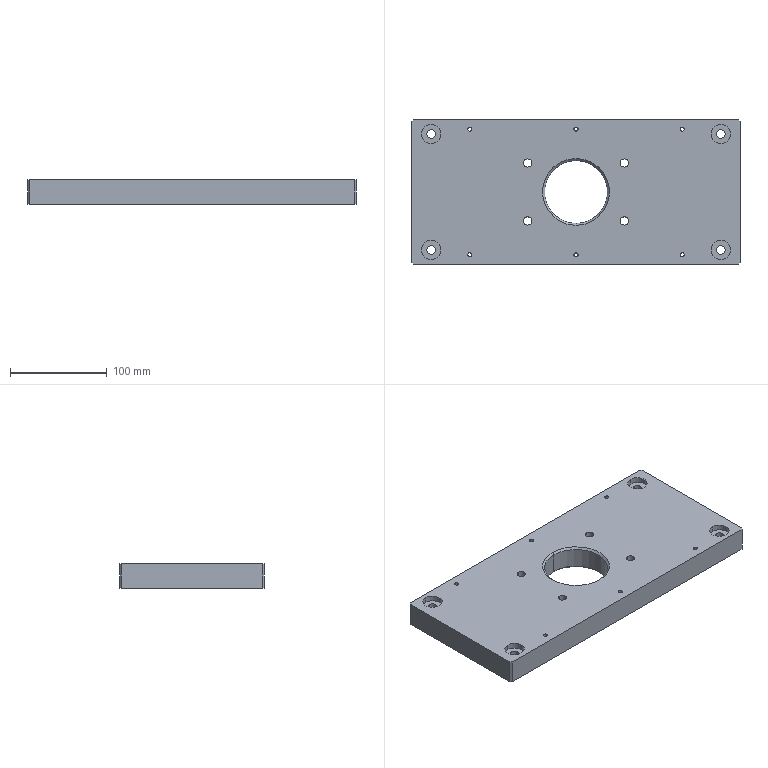Part | 1 solid | 56 faces | box 340 x 150 x 25 mm | volume 1170368 mm3 | cylinder 38 | plane 14 | cone 4 | commonest cylinder face diameters 4.2 x12 8.5 x8 9 x8 20 x8 65.2 x2